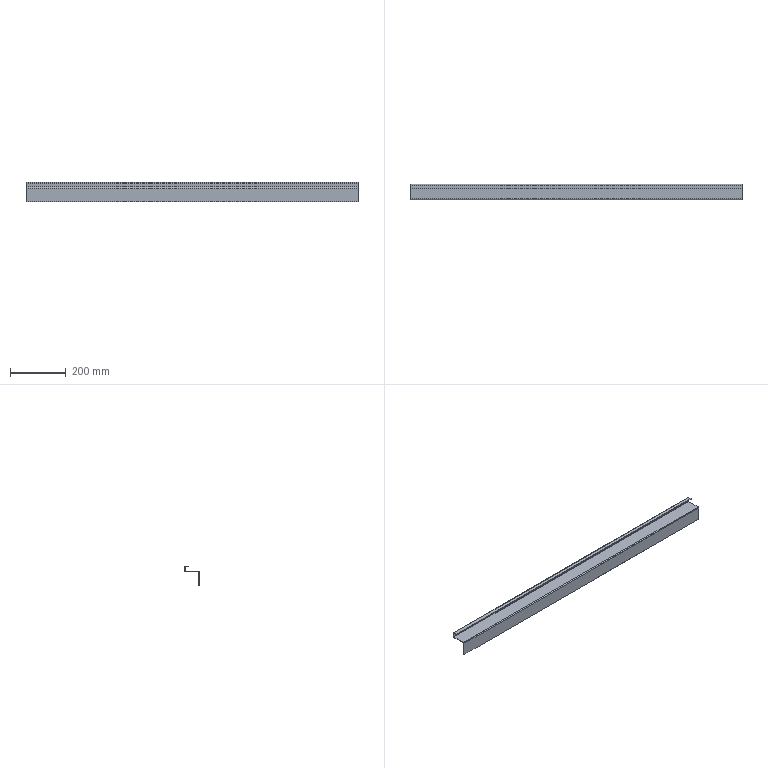Part | SolidWorks | features BaseBody 1 | 1 solid | 30 faces | box 1186 x 54 x 70 mm | volume 314112 mm3 | plane 24 | cylinder 6 | commonest cylinder face diameters 2 x3 6 x3
STEP:
#1=CARTESIAN_POINT('',(-593.,12.,16.));
#2=VERTEX_POINT('',#1);
#3=CARTESIAN_POINT('',(593.,12.,16.));
#4=VERTEX_POINT('',#3);
#5=CARTESIAN_POINT('',(593.,12.,16.));
#6=DIRECTION('',(1.,0.,0.));
#7=VECTOR('',#6,1000.);
#8=LINE('',#5,#7);
#9=EDGE_CURVE('',#2,#4,#8,.T.);
#10=ORIENTED_EDGE('',*,*,#9,.T.);
#11=CARTESIAN_POINT('',(593.,12.,18.));
#12=VERTEX_POINT('',#11);
#13=CARTESIAN_POINT('',(593.,12.,18.));
#14=DIRECTION('',(0.,0.,-1.));
#15=VECTOR('',#14,1000.);
#16=LINE('',#13,#15);
#17=EDGE_CURVE('',#12,#4,#16,.T.);
#18=ORIENTED_EDGE('',*,*,#17,.F.);
#19=CARTESIAN_POINT('',(-593.,12.,18.));
#20=VERTEX_POINT('',#19);
#21=CARTESIAN_POINT('',(0.,12.,18.));
#22=DIRECTION('',(1.,0.,0.));
#23=VECTOR('',#22,1000.);
#24=LINE('',#21,#23);
#25=EDGE_CURVE('',#20,#12,#24,.T.);
#26=ORIENTED_EDGE('',*,*,#25,.F.);
#27=CARTESIAN_POINT('',(-593.,12.,18.));
#28=DIRECTION('',(0.,0.,-1.));
#29=VECTOR('',#28,1000.);
#30=LINE('',#27,#29);
#31=EDGE_CURVE('',#20,#2,#30,.T.);
#32=ORIENTED_EDGE('',*,*,#31,.T.);
#33=EDGE_LOOP('',(#10,#18,#26,#32));
#34=FACE_OUTER_BOUND('',#33,.T.);
#35=CARTESIAN_POINT('',(593.,12.,18.));
#36=DIRECTION('',(0.,1.,0.));
#37=DIRECTION('',(0.,0.,-1.));
#38=AXIS2_PLACEMENT_3D('',#35,#36,#37);
#39=PLANE('',#38);
#40=ADVANCED_FACE('',(#34),#39,.F.);
#41=CARTESIAN_POINT('',(-593.,24.,16.));
#42=VERTEX_POINT('',#41);
#43=CARTESIAN_POINT('',(-593.,12.,16.));
#44=DIRECTION('',(0.,-1.,0.));
#45=VECTOR('',#44,1000.);
#46=LINE('',#43,#45);
#47=EDGE_CURVE('',#42,#2,#46,.T.);
#48=ORIENTED_EDGE('',*,*,#47,.F.);
#49=CARTESIAN_POINT('',(593.,24.,16.));
#50=VERTEX_POINT('',#49);
#51=CARTESIAN_POINT('',(593.,24.,16.));
#52=DIRECTION('',(-1.,0.,0.));
#53=VECTOR('',#52,1000.);
#54=LINE('',#51,#53);
#55=EDGE_CURVE('',#50,#42,#54,.T.);
#56=ORIENTED_EDGE('',*,*,#55,.F.);
#57=CARTESIAN_POINT('',(593.,25.,16.));
#58=DIRECTION('',(0.,1.,0.));
#59=VECTOR('',#58,1000.);
#60=LINE('',#57,#59);
#61=EDGE_CURVE('',#4,#50,#60,.T.);
#62=ORIENTED_EDGE('',*,*,#61,.F.);
#63=ORIENTED_EDGE('',*,*,#9,.F.);
#64=EDGE_LOOP('',(#48,#56,#62,#63));
#65=FACE_OUTER_BOUND('',#64,.T.);
#66=CARTESIAN_POINT('',(0.,0.,16.));
#67=DIRECTION('',(0.,0.,-1.));
#68=DIRECTION('',(0.,-1.,0.));
#69=AXIS2_PLACEMENT_3D('',#66,#67,#68);
#70=PLANE('',#69);
#71=ADVANCED_FACE('',(#65),#70,.T.);
#72=CARTESIAN_POINT('',(-593.,24.,18.));
#73=VERTEX_POINT('',#72);
#74=CARTESIAN_POINT('',(593.,24.,18.));
#75=VERTEX_POINT('',#74);
#76=CARTESIAN_POINT('',(593.,24.,18.));
#77=DIRECTION('',(1.,0.,0.));
#78=VECTOR('',#77,1000.);
#79=LINE('',#76,#78);
#80=EDGE_CURVE('',#73,#75,#79,.T.);
#81=ORIENTED_EDGE('',*,*,#80,.F.);
#82=CARTESIAN_POINT('',(-593.,0.,18.));
#83=DIRECTION('',(0.,-1.,0.));
#84=VECTOR('',#83,1000.);
#85=LINE('',#82,#84);
#86=EDGE_CURVE('',#73,#20,#85,.T.);
#87=ORIENTED_EDGE('',*,*,#86,.T.);
#88=ORIENTED_EDGE('',*,*,#25,.T.);
#89=CARTESIAN_POINT('',(593.,0.,18.));
#90=DIRECTION('',(0.,1.,0.));
#91=VECTOR('',#90,1000.);
#92=LINE('',#89,#91);
#93=EDGE_CURVE('',#12,#75,#92,.T.);
#94=ORIENTED_EDGE('',*,*,#93,.T.);
#95=EDGE_LOOP('',(#81,#87,#88,#94));
#96=FACE_OUTER_BOUND('',#95,.T.);
#97=CARTESIAN_POINT('',(0.,0.,18.));
#98=DIRECTION('',(0.,0.,-1.));
#99=DIRECTION('',(0.,-1.,0.));
#100=AXIS2_PLACEMENT_3D('',#97,#98,#99);
#101=PLANE('',#100);
#102=ADVANCED_FACE('',(#96),#101,.F.);
#103=CARTESIAN_POINT('',(-593.,24.,16.));
#104=DIRECTION('',(0.,0.,1.));
#105=VECTOR('',#104,1000.);
#106=LINE('',#103,#105);
#107=EDGE_CURVE('',#42,#73,#106,.T.);
#108=ORIENTED_EDGE('',*,*,#107,.F.);
#109=ORIENTED_EDGE('',*,*,#47,.T.);
#110=ORIENTED_EDGE('',*,*,#31,.F.);
#111=ORIENTED_EDGE('',*,*,#86,.F.);
#112=EDGE_LOOP('',(#108,#109,#110,#111));
#113=FACE_OUTER_BOUND('',#112,.T.);
#114=CARTESIAN_POINT('',(-593.,12.,18.));
#115=DIRECTION('',(1.,0.,0.));
#116=DIRECTION('',(0.,0.,1.));
#117=AXIS2_PLACEMENT_3D('',#114,#115,#116);
#118=PLANE('',#117);
#119=ADVANCED_FACE('',(#113),#118,.F.);
#120=CARTESIAN_POINT('',(593.,24.,18.));
#121=DIRECTION('',(0.,0.,1.));
#122=VECTOR('',#121,1000.);
#123=LINE('',#120,#122);
#124=EDGE_CURVE('',#50,#75,#123,.T.);
#125=ORIENTED_EDGE('',*,*,#124,.T.);
#126=ORIENTED_EDGE('',*,*,#93,.F.);
#127=ORIENTED_EDGE('',*,*,#17,.T.);
#128=ORIENTED_EDGE('',*,*,#61,.T.);
#129=EDGE_LOOP('',(#125,#126,#127,#128));
#130=FACE_OUTER_BOUND('',#129,.T.);
#131=CARTESIAN_POINT('',(593.,25.,18.));
#132=DIRECTION('',(-1.,0.,0.));
#133=DIRECTION('',(0.,0.,1.));
#134=AXIS2_PLACEMENT_3D('',#131,#132,#133);
#135=PLANE('',#134);
#136=ADVANCED_FACE('',(#130),#135,.F.);
#137=CARTESIAN_POINT('',(-593.,25.,15.));
#138=VERTEX_POINT('',#137);
#139=CARTESIAN_POINT('',(593.,25.,15.));
#140=VERTEX_POINT('',#139);
#141=CARTESIAN_POINT('',(-593.,25.,15.));
#142=DIRECTION('',(1.,0.,0.));
#143=VECTOR('',#142,1000.);
#144=LINE('',#141,#143);
#145=EDGE_CURVE('',#138,#140,#144,.T.);
#146=ORIENTED_EDGE('',*,*,#145,.T.);
#147=CARTESIAN_POINT('',(593.,24.,15.));
#148=DIRECTION('',(1.,0.,0.));
#149=DIRECTION('',(0.,0.,1.));
#150=AXIS2_PLACEMENT_3D('',#147,#148,#149);
#151=CIRCLE('',#150,1.);
#152=EDGE_CURVE('',#140,#50,#151,.T.);
#153=ORIENTED_EDGE('',*,*,#152,.T.);
#154=ORIENTED_EDGE('',*,*,#55,.T.);
#155=CARTESIAN_POINT('',(-593.,24.,15.));
#156=DIRECTION('',(-1.,0.,0.));
#157=DIRECTION('',(0.,0.,1.));
#158=AXIS2_PLACEMENT_3D('',#155,#156,#157);
#159=CIRCLE('',#158,1.);
#160=EDGE_CURVE('',#42,#138,#159,.T.);
#161=ORIENTED_EDGE('',*,*,#160,.T.);
#162=EDGE_LOOP('',(#146,#153,#154,#161));
#163=FACE_OUTER_BOUND('',#162,.T.);
#164=CARTESIAN_POINT('',(-593.,24.,15.));
#165=DIRECTION('',(-1.,0.,0.));
#166=DIRECTION('',(0.,0.,1.));
#167=AXIS2_PLACEMENT_3D('',#164,#165,#166);
#168=CYLINDRICAL_SURFACE('',#167,1.);
#169=ADVANCED_FACE('',(#163),#168,.F.);
#170=CARTESIAN_POINT('',(-593.,27.,15.));
#171=VERTEX_POINT('',#170);
#172=CARTESIAN_POINT('',(593.,27.,15.));
#173=VERTEX_POINT('',#172);
#174=CARTESIAN_POINT('',(-593.,27.,15.));
#175=DIRECTION('',(1.,0.,0.));
#176=VECTOR('',#175,1000.);
#177=LINE('',#174,#176);
#178=EDGE_CURVE('',#171,#173,#177,.T.);
#179=ORIENTED_EDGE('',*,*,#178,.F.);
#180=CARTESIAN_POINT('',(-593.,24.,15.));
#181=DIRECTION('',(-1.,0.,0.));
#182=DIRECTION('',(0.,0.,1.));
#183=AXIS2_PLACEMENT_3D('',#180,#181,#182);
#184=CIRCLE('',#183,3.);
#185=EDGE_CURVE('',#73,#171,#184,.T.);
#186=ORIENTED_EDGE('',*,*,#185,.F.);
#187=ORIENTED_EDGE('',*,*,#80,.T.);
#188=CARTESIAN_POINT('',(593.,24.,15.));
#189=DIRECTION('',(1.,0.,0.));
#190=DIRECTION('',(0.,0.,1.));
#191=AXIS2_PLACEMENT_3D('',#188,#189,#190);
#192=CIRCLE('',#191,3.);
#193=EDGE_CURVE('',#173,#75,#192,.T.);
#194=ORIENTED_EDGE('',*,*,#193,.F.);
#195=EDGE_LOOP('',(#179,#186,#187,#194));
#196=FACE_OUTER_BOUND('',#195,.T.);
#197=CARTESIAN_POINT('',(-593.,24.,15.));
#198=DIRECTION('',(-1.,0.,0.));
#199=DIRECTION('',(0.,0.,1.));
#200=AXIS2_PLACEMENT_3D('',#197,#198,#199);
#201=CYLINDRICAL_SURFACE('',#200,3.);
#202=ADVANCED_FACE('',(#196),#201,.T.);
#203=ORIENTED_EDGE('',*,*,#160,.F.);
#204=ORIENTED_EDGE('',*,*,#107,.T.);
#205=ORIENTED_EDGE('',*,*,#185,.T.);
#206=CARTESIAN_POINT('',(-593.,25.,15.));
#207=DIRECTION('',(0.,1.,0.));
#208=VECTOR('',#207,1000.);
#209=LINE('',#206,#208);
#210=EDGE_CURVE('',#138,#171,#209,.T.);
#211=ORIENTED_EDGE('',*,*,#210,.F.);
#212=EDGE_LOOP('',(#203,#204,#205,#211));
#213=FACE_OUTER_BOUND('',#212,.T.);
#214=CARTESIAN_POINT('',(-593.,24.,15.));
#215=DIRECTION('',(1.,0.,0.));
#216=DIRECTION('',(0.,1.,0.));
#217=AXIS2_PLACEMENT_3D('',#214,#215,#216);
#218=PLANE('',#217);
#219=ADVANCED_FACE('',(#213),#218,.F.);
#220=ORIENTED_EDGE('',*,*,#124,.F.);
#221=ORIENTED_EDGE('',*,*,#152,.F.);
#222=CARTESIAN_POINT('',(593.,25.,15.));
#223=DIRECTION('',(0.,1.,0.));
#224=VECTOR('',#223,1000.);
#225=LINE('',#222,#224);
#226=EDGE_CURVE('',#140,#173,#225,.T.);
#227=ORIENTED_EDGE('',*,*,#226,.T.);
#228=ORIENTED_EDGE('',*,*,#193,.T.);
#229=EDGE_LOOP('',(#220,#221,#227,#228));
#230=FACE_OUTER_BOUND('',#229,.T.);
#231=CARTESIAN_POINT('',(593.,24.,15.));
#232=DIRECTION('',(1.,0.,0.));
#233=DIRECTION('',(0.,1.,0.));
#234=AXIS2_PLACEMENT_3D('',#231,#232,#233);
#235=PLANE('',#234);
#236=ADVANCED_FACE('',(#230),#235,.T.);
#237=ORIENTED_EDGE('',*,*,#226,.F.);
#238=CARTESIAN_POINT('',(593.,25.,1.));
#239=VERTEX_POINT('',#238);
#240=CARTESIAN_POINT('',(593.,25.,0.));
#241=DIRECTION('',(0.,0.,1.));
#242=VECTOR('',#241,1000.);
#243=LINE('',#240,#242);
#244=EDGE_CURVE('',#239,#140,#243,.T.);
#245=ORIENTED_EDGE('',*,*,#244,.F.);
#246=CARTESIAN_POINT('',(593.,27.,1.));
#247=VERTEX_POINT('',#246);
#248=CARTESIAN_POINT('',(593.,27.,1.));
#249=DIRECTION('',(0.,1.,0.));
#250=VECTOR('',#249,1000.);
#251=LINE('',#248,#250);
#252=EDGE_CURVE('',#239,#247,#251,.T.);
#253=ORIENTED_EDGE('',*,*,#252,.T.);
#254=CARTESIAN_POINT('',(593.,27.,18.));
#255=DIRECTION('',(0.,0.,1.));
#256=VECTOR('',#255,1000.);
#257=LINE('',#254,#256);
#258=EDGE_CURVE('',#247,#173,#257,.T.);
#259=ORIENTED_EDGE('',*,*,#258,.T.);
#260=EDGE_LOOP('',(#237,#245,#253,#259));
#261=FACE_OUTER_BOUND('',#260,.T.);
#262=CARTESIAN_POINT('',(593.,27.,18.));
#263=DIRECTION('',(1.,0.,0.));
#264=DIRECTION('',(0.,1.,0.));
#265=AXIS2_PLACEMENT_3D('',#262,#263,#264);
#266=PLANE('',#265);
#267=ADVANCED_FACE('',(#261),#266,.T.);
#268=CARTESIAN_POINT('',(-593.,24.,0.));
#269=VERTEX_POINT('',#268);
#270=CARTESIAN_POINT('',(593.,24.,0.));
#271=VERTEX_POINT('',#270);
#272=CARTESIAN_POINT('',(-593.,24.,0.));
#273=DIRECTION('',(1.,0.,0.));
#274=VECTOR('',#273,1000.);
#275=LINE('',#272,#274);
#276=EDGE_CURVE('',#269,#271,#275,.T.);
#277=ORIENTED_EDGE('',*,*,#276,.T.);
#278=CARTESIAN_POINT('',(593.,24.,1.));
#279=DIRECTION('',(1.,0.,0.));
#280=DIRECTION('',(0.,0.,1.));
#281=AXIS2_PLACEMENT_3D('',#278,#279,#280);
#282=CIRCLE('',#281,1.);
#283=EDGE_CURVE('',#271,#239,#282,.T.);
#284=ORIENTED_EDGE('',*,*,#283,.T.);
#285=CARTESIAN_POINT('',(-593.,25.,1.));
#286=VERTEX_POINT('',#285);
#287=CARTESIAN_POINT('',(593.,25.,1.));
#288=DIRECTION('',(-1.,0.,0.));
#289=VECTOR('',#288,1000.);
#290=LINE('',#287,#289);
#291=EDGE_CURVE('',#239,#286,#290,.T.);
#292=ORIENTED_EDGE('',*,*,#291,.T.);
#293=CARTESIAN_POINT('',(-593.,24.,1.));
#294=DIRECTION('',(-1.,0.,0.));
#295=DIRECTION('',(0.,0.,1.));
#296=AXIS2_PLACEMENT_3D('',#293,#294,#295);
#297=CIRCLE('',#296,1.);
#298=EDGE_CURVE('',#286,#269,#297,.T.);
#299=ORIENTED_EDGE('',*,*,#298,.T.);
#300=EDGE_LOOP('',(#277,#284,#292,#299));
#301=FACE_OUTER_BOUND('',#300,.T.);
#302=CARTESIAN_POINT('',(-593.,24.,1.));
#303=DIRECTION('',(-1.,0.,0.));
#304=DIRECTION('',(0.,1.,0.));
#305=AXIS2_PLACEMENT_3D('',#302,#303,#304);
#306=CYLINDRICAL_SURFACE('',#305,1.);
#307=ADVANCED_FACE('',(#301),#306,.F.);
#308=CARTESIAN_POINT('',(-593.,24.,-2.));
#309=VERTEX_POINT('',#308);
#310=CARTESIAN_POINT('',(593.,24.,-2.));
#311=VERTEX_POINT('',#310);
#312=CARTESIAN_POINT('',(-593.,24.,-2.));
#313=DIRECTION('',(1.,0.,0.));
#314=VECTOR('',#313,1000.);
#315=LINE('',#312,#314);
#316=EDGE_CURVE('',#309,#311,#315,.T.);
#317=ORIENTED_EDGE('',*,*,#316,.F.);
#318=CARTESIAN_POINT('',(-593.,27.,1.));
#319=VERTEX_POINT('',#318);
#320=CARTESIAN_POINT('',(-593.,24.,1.));
#321=DIRECTION('',(-1.,0.,0.));
#322=DIRECTION('',(0.,0.,1.));
#323=AXIS2_PLACEMENT_3D('',#320,#321,#322);
#324=CIRCLE('',#323,3.);
#325=EDGE_CURVE('',#319,#309,#324,.T.);
#326=ORIENTED_EDGE('',*,*,#325,.F.);
#327=CARTESIAN_POINT('',(0.,27.,1.));
#328=DIRECTION('',(-1.,0.,0.));
#329=VECTOR('',#328,1000.);
#330=LINE('',#327,#329);
#331=EDGE_CURVE('',#247,#319,#330,.T.);
#332=ORIENTED_EDGE('',*,*,#331,.F.);
#333=CARTESIAN_POINT('',(593.,24.,1.));
#334=DIRECTION('',(1.,0.,0.));
#335=DIRECTION('',(0.,0.,1.));
#336=AXIS2_PLACEMENT_3D('',#333,#334,#335);
#337=CIRCLE('',#336,3.);
#338=EDGE_CURVE('',#311,#247,#337,.T.);
#339=ORIENTED_EDGE('',*,*,#338,.F.);
#340=EDGE_LOOP('',(#317,#326,#332,#339));
#341=FACE_OUTER_BOUND('',#340,.T.);
#342=CARTESIAN_POINT('',(-593.,24.,1.));
#343=DIRECTION('',(-1.,0.,0.));
#344=DIRECTION('',(0.,1.,0.));
#345=AXIS2_PLACEMENT_3D('',#342,#343,#344);
#346=CYLINDRICAL_SURFACE('',#345,3.);
#347=ADVANCED_FACE('',(#341),#346,.T.);
#348=ORIENTED_EDGE('',*,*,#298,.F.);
#349=CARTESIAN_POINT('',(-593.,25.,1.));
#350=DIRECTION('',(0.,1.,0.));
#351=VECTOR('',#350,1000.);
#352=LINE('',#349,#351);
#353=EDGE_CURVE('',#286,#319,#352,.T.);
#354=ORIENTED_EDGE('',*,*,#353,.T.);
#355=ORIENTED_EDGE('',*,*,#325,.T.);
#356=CARTESIAN_POINT('',(-593.,24.,0.));
#357=DIRECTION('',(0.,0.,-1.));
#358=VECTOR('',#357,1000.);
#359=LINE('',#356,#358);
#360=EDGE_CURVE('',#269,#309,#359,.T.);
#361=ORIENTED_EDGE('',*,*,#360,.F.);
#362=EDGE_LOOP('',(#348,#354,#355,#361));
#363=FACE_OUTER_BOUND('',#362,.T.);
#364=CARTESIAN_POINT('',(-593.,24.,1.));
#365=DIRECTION('',(1.,0.,0.));
#366=DIRECTION('',(0.,1.,0.));
#367=AXIS2_PLACEMENT_3D('',#364,#365,#366);
#368=PLANE('',#367);
#369=ADVANCED_FACE('',(#363),#368,.F.);
#370=ORIENTED_EDGE('',*,*,#252,.F.);
#371=ORIENTED_EDGE('',*,*,#283,.F.);
#372=CARTESIAN_POINT('',(593.,24.,0.));
#373=DIRECTION('',(0.,0.,-1.));
#374=VECTOR('',#373,1000.);
#375=LINE('',#372,#374);
#376=EDGE_CURVE('',#271,#311,#375,.T.);
#377=ORIENTED_EDGE('',*,*,#376,.T.);
#378=ORIENTED_EDGE('',*,*,#338,.T.);
#379=EDGE_LOOP('',(#370,#371,#377,#378));
#380=FACE_OUTER_BOUND('',#379,.T.);
#381=CARTESIAN_POINT('',(593.,24.,1.));
#382=DIRECTION('',(1.,0.,0.));
#383=DIRECTION('',(0.,1.,0.));
#384=AXIS2_PLACEMENT_3D('',#381,#382,#383);
#385=PLANE('',#384);
#386=ADVANCED_FACE('',(#380),#385,.T.);
#387=CARTESIAN_POINT('',(-593.,-25.,-52.));
#388=VERTEX_POINT('',#387);
#389=CARTESIAN_POINT('',(593.,-25.,-52.));
#390=VERTEX_POINT('',#389);
#391=CARTESIAN_POINT('',(593.,-25.,-52.));
#392=DIRECTION('',(1.,0.,0.));
#393=VECTOR('',#392,1000.);
#394=LINE('',#391,#393);
#395=EDGE_CURVE('',#388,#390,#394,.T.);
#396=ORIENTED_EDGE('',*,*,#395,.T.);
#397=CARTESIAN_POINT('',(593.,-27.,-52.));
#398=VERTEX_POINT('',#397);
#399=CARTESIAN_POINT('',(593.,-27.,-52.));
#400=DIRECTION('',(0.,1.,0.));
#401=VECTOR('',#400,1000.);
#402=LINE('',#399,#401);
#403=EDGE_CURVE('',#398,#390,#402,.T.);
#404=ORIENTED_EDGE('',*,*,#403,.F.);
#405=CARTESIAN_POINT('',(-593.,-27.,-52.));
#406=VERTEX_POINT('',#405);
#407=CARTESIAN_POINT('',(0.,-27.,-52.));
#408=DIRECTION('',(1.,0.,0.));
#409=VECTOR('',#408,1000.);
#410=LINE('',#407,#409);
#411=EDGE_CURVE('',#406,#398,#410,.T.);
#412=ORIENTED_EDGE('',*,*,#411,.F.);
#413=CARTESIAN_POINT('',(-593.,-27.,-52.));
#414=DIRECTION('',(0.,1.,0.));
#415=VECTOR('',#414,1000.);
#416=LINE('',#413,#415);
#417=EDGE_CURVE('',#406,#388,#416,.T.);
#418=ORIENTED_EDGE('',*,*,#417,.T.);
#419=EDGE_LOOP('',(#396,#404,#412,#418));
#420=FACE_OUTER_BOUND('',#419,.T.);
#421=CARTESIAN_POINT('',(593.,-27.,-52.));
#422=DIRECTION('',(0.,0.,1.));
#423=DIRECTION('',(0.,-1.,0.));
#424=AXIS2_PLACEMENT_3D('',#421,#422,#423);
#425=PLANE('',#424);
#426=ADVANCED_FACE('',(#420),#425,.F.);
#427=CARTESIAN_POINT('',(-593.,-25.,-3.));
#428=VERTEX_POINT('',#427);
#429=CARTESIAN_POINT('',(-593.,-25.,-52.));
#430=DIRECTION('',(0.,0.,-1.));
#431=VECTOR('',#430,1000.);
#432=LINE('',#429,#431);
#433=EDGE_CURVE('',#428,#388,#432,.T.);
#434=ORIENTED_EDGE('',*,*,#433,.F.);
#435=CARTESIAN_POINT('',(593.,-25.,-3.));
#436=VERTEX_POINT('',#435);
#437=CARTESIAN_POINT('',(593.,-25.,-3.));
#438=DIRECTION('',(-1.,0.,0.));
#439=VECTOR('',#438,1000.);
#440=LINE('',#437,#439);
#441=EDGE_CURVE('',#436,#428,#440,.T.);
#442=ORIENTED_EDGE('',*,*,#441,.F.);
#443=CARTESIAN_POINT('',(593.,-25.,-2.));
#444=DIRECTION('',(0.,0.,1.));
#445=VECTOR('',#444,1000.);
#446=LINE('',#443,#445);
#447=EDGE_CURVE('',#390,#436,#446,.T.);
#448=ORIENTED_EDGE('',*,*,#447,.F.);
#449=ORIENTED_EDGE('',*,*,#395,.F.);
#450=EDGE_LOOP('',(#434,#442,#448,#449));
#451=FACE_OUTER_BOUND('',#450,.T.);
#452=CARTESIAN_POINT('',(0.,-25.,0.));
#453=DIRECTION('',(0.,1.,0.));
#454=DIRECTION('',(0.,0.,-1.));
#455=AXIS2_PLACEMENT_3D('',#452,#453,#454);
#456=PLANE('',#455);
#457=ADVANCED_FACE('',(#451),#456,.T.);
#458=CARTESIAN_POINT('',(-593.,-27.,-3.));
#459=VERTEX_POINT('',#458);
#460=CARTESIAN_POINT('',(593.,-27.,-3.));
#461=VERTEX_POINT('',#460);
#462=CARTESIAN_POINT('',(593.,-27.,-3.));
#463=DIRECTION('',(1.,0.,0.));
#464=VECTOR('',#463,1000.);
#465=LINE('',#462,#464);
#466=EDGE_CURVE('',#459,#461,#465,.T.);
#467=ORIENTED_EDGE('',*,*,#466,.F.);
#468=CARTESIAN_POINT('',(-593.,-27.,0.));
#469=DIRECTION('',(0.,0.,-1.));
#470=VECTOR('',#469,1000.);
#471=LINE('',#468,#470);
#472=EDGE_CURVE('',#459,#406,#471,.T.);
#473=ORIENTED_EDGE('',*,*,#472,.T.);
#474=ORIENTED_EDGE('',*,*,#411,.T.);
#475=CARTESIAN_POINT('',(593.,-27.,0.));
#476=DIRECTION('',(0.,0.,1.));
#477=VECTOR('',#476,1000.);
#478=LINE('',#475,#477);
#479=EDGE_CURVE('',#398,#461,#478,.T.);
#480=ORIENTED_EDGE('',*,*,#479,.T.);
#481=EDGE_LOOP('',(#467,#473,#474,#480));
#482=FACE_OUTER_BOUND('',#481,.T.);
#483=CARTESIAN_POINT('',(0.,-27.,0.));
#484=DIRECTION('',(0.,1.,0.));
#485=DIRECTION('',(0.,0.,-1.));
#486=AXIS2_PLACEMENT_3D('',#483,#484,#485);
#487=PLANE('',#486);
#488=ADVANCED_FACE('',(#482),#487,.F.);
#489=CARTESIAN_POINT('',(593.,-27.,-3.));
#490=DIRECTION('',(0.,-1.,0.));
#491=VECTOR('',#490,1000.);
#492=LINE('',#489,#491);
#493=EDGE_CURVE('',#436,#461,#492,.T.);
#494=ORIENTED_EDGE('',*,*,#493,.T.);
#495=ORIENTED_EDGE('',*,*,#479,.F.);
#496=ORIENTED_EDGE('',*,*,#403,.T.);
#497=ORIENTED_EDGE('',*,*,#447,.T.);
#498=EDGE_LOOP('',(#494,#495,#496,#497));
#499=FACE_OUTER_BOUND('',#498,.T.);
#500=CARTESIAN_POINT('',(593.,-27.,-2.));
#501=DIRECTION('',(-1.,0.,0.));
#502=DIRECTION('',(0.,1.,0.));
#503=AXIS2_PLACEMENT_3D('',#500,#501,#502);
#504=PLANE('',#503);
#505=ADVANCED_FACE('',(#499),#504,.F.);
#506=CARTESIAN_POINT('',(-593.,-25.,-3.));
#507=DIRECTION('',(0.,-1.,0.));
#508=VECTOR('',#507,1000.);
#509=LINE('',#506,#508);
#510=EDGE_CURVE('',#428,#459,#509,.T.);
#511=ORIENTED_EDGE('',*,*,#510,.F.);
#512=ORIENTED_EDGE('',*,*,#433,.T.);
#513=ORIENTED_EDGE('',*,*,#417,.F.);
#514=ORIENTED_EDGE('',*,*,#472,.F.);
#515=EDGE_LOOP('',(#511,#512,#513,#514));
#516=FACE_OUTER_BOUND('',#515,.T.);
#517=CARTESIAN_POINT('',(-593.,-27.,-52.));
#518=DIRECTION('',(1.,0.,0.));
#519=DIRECTION('',(0.,1.,0.));
#520=AXIS2_PLACEMENT_3D('',#517,#518,#519);
#521=PLANE('',#520);
#522=ADVANCED_FACE('',(#516),#521,.F.);
#523=CARTESIAN_POINT('',(-593.,-24.,-2.));
#524=VERTEX_POINT('',#523);
#525=CARTESIAN_POINT('',(593.,-24.,-2.));
#526=VERTEX_POINT('',#525);
#527=CARTESIAN_POINT('',(-593.,-24.,-2.));
#528=DIRECTION('',(1.,0.,0.));
#529=VECTOR('',#528,1000.);
#530=LINE('',#527,#529);
#531=EDGE_CURVE('',#524,#526,#530,.T.);
#532=ORIENTED_EDGE('',*,*,#531,.T.);
#533=CARTESIAN_POINT('',(593.,-24.,-3.));
#534=DIRECTION('',(1.,0.,0.));
#535=DIRECTION('',(0.,0.,1.));
#536=AXIS2_PLACEMENT_3D('',#533,#534,#535);
#537=CIRCLE('',#536,1.);
#538=EDGE_CURVE('',#526,#436,#537,.T.);
#539=ORIENTED_EDGE('',*,*,#538,.T.);
#540=ORIENTED_EDGE('',*,*,#441,.T.);
#541=CARTESIAN_POINT('',(-593.,-24.,-3.));
#542=DIRECTION('',(-1.,0.,0.));
#543=DIRECTION('',(0.,0.,1.));
#544=AXIS2_PLACEMENT_3D('',#541,#542,#543);
#545=CIRCLE('',#544,1.);
#546=EDGE_CURVE('',#428,#524,#545,.T.);
#547=ORIENTED_EDGE('',*,*,#546,.T.);
#548=EDGE_LOOP('',(#532,#539,#540,#547));
#549=FACE_OUTER_BOUND('',#548,.T.);
#550=CARTESIAN_POINT('',(-593.,-24.,-3.));
#551=DIRECTION('',(-1.,0.,0.));
#552=DIRECTION('',(0.,-1.,0.));
#553=AXIS2_PLACEMENT_3D('',#550,#551,#552);
#554=CYLINDRICAL_SURFACE('',#553,1.);
#555=ADVANCED_FACE('',(#549),#554,.F.);
#556=CARTESIAN_POINT('',(-593.,-24.,0.));
#557=VERTEX_POINT('',#556);
#558=CARTESIAN_POINT('',(593.,-24.,0.));
#559=VERTEX_POINT('',#558);
#560=CARTESIAN_POINT('',(-593.,-24.,0.));
#561=DIRECTION('',(1.,0.,0.));
#562=VECTOR('',#561,1000.);
#563=LINE('',#560,#562);
#564=EDGE_CURVE('',#557,#559,#563,.T.);
#565=ORIENTED_EDGE('',*,*,#564,.F.);
#566=CARTESIAN_POINT('',(-593.,-24.,-3.));
#567=DIRECTION('',(-1.,0.,0.));
#568=DIRECTION('',(0.,0.,1.));
#569=AXIS2_PLACEMENT_3D('',#566,#567,#568);
#570=CIRCLE('',#569,3.);
#571=EDGE_CURVE('',#459,#557,#570,.T.);
#572=ORIENTED_EDGE('',*,*,#571,.F.);
#573=ORIENTED_EDGE('',*,*,#466,.T.);
#574=CARTESIAN_POINT('',(593.,-24.,-3.));
#575=DIRECTION('',(1.,0.,0.));
#576=DIRECTION('',(0.,0.,1.));
#577=AXIS2_PLACEMENT_3D('',#574,#575,#576);
#578=CIRCLE('',#577,3.);
#579=EDGE_CURVE('',#559,#461,#578,.T.);
#580=ORIENTED_EDGE('',*,*,#579,.F.);
#581=EDGE_LOOP('',(#565,#572,#573,#580));
#582=FACE_OUTER_BOUND('',#581,.T.);
#583=CARTESIAN_POINT('',(-593.,-24.,-3.));
#584=DIRECTION('',(-1.,0.,0.));
#585=DIRECTION('',(0.,-1.,0.));
#586=AXIS2_PLACEMENT_3D('',#583,#584,#585);
#587=CYLINDRICAL_SURFACE('',#586,3.);
#588=ADVANCED_FACE('',(#582),#587,.T.);
#589=ORIENTED_EDGE('',*,*,#546,.F.);
#590=ORIENTED_EDGE('',*,*,#510,.T.);
#591=ORIENTED_EDGE('',*,*,#571,.T.);
#592=CARTESIAN_POINT('',(-593.,-24.,-2.));
#593=DIRECTION('',(0.,0.,1.));
#594=VECTOR('',#593,1000.);
#595=LINE('',#592,#594);
#596=EDGE_CURVE('',#524,#557,#595,.T.);
#597=ORIENTED_EDGE('',*,*,#596,.F.);
#598=EDGE_LOOP('',(#589,#590,#591,#597));
#599=FACE_OUTER_BOUND('',#598,.T.);
#600=CARTESIAN_POINT('',(-593.,-24.,-3.));
#601=DIRECTION('',(1.,0.,0.));
#602=DIRECTION('',(0.,1.,0.));
#603=AXIS2_PLACEMENT_3D('',#600,#601,#602);
#604=PLANE('',#603);
#605=ADVANCED_FACE('',(#599),#604,.F.);
#606=ORIENTED_EDGE('',*,*,#493,.F.);
#607=ORIENTED_EDGE('',*,*,#538,.F.);
#608=CARTESIAN_POINT('',(593.,-24.,-2.));
#609=DIRECTION('',(0.,0.,1.));
#610=VECTOR('',#609,1000.);
#611=LINE('',#608,#610);
#612=EDGE_CURVE('',#526,#559,#611,.T.);
#613=ORIENTED_EDGE('',*,*,#612,.T.);
#614=ORIENTED_EDGE('',*,*,#579,.T.);
#615=EDGE_LOOP('',(#606,#607,#613,#614));
#616=FACE_OUTER_BOUND('',#615,.T.);
#617=CARTESIAN_POINT('',(593.,-24.,-3.));
#618=DIRECTION('',(1.,0.,0.));
#619=DIRECTION('',(0.,1.,0.));
#620=AXIS2_PLACEMENT_3D('',#617,#618,#619);
#621=PLANE('',#620);
#622=ADVANCED_FACE('',(#616),#621,.T.);
#623=ORIENTED_EDGE('',*,*,#376,.F.);
#624=CARTESIAN_POINT('',(593.,27.,0.));
#625=DIRECTION('',(0.,1.,0.));
#626=VECTOR('',#625,1000.);
#627=LINE('',#624,#626);
#628=EDGE_CURVE('',#559,#271,#627,.T.);
#629=ORIENTED_EDGE('',*,*,#628,.F.);
#630=ORIENTED_EDGE('',*,*,#612,.F.);
#631=CARTESIAN_POINT('',(593.,27.,-2.));
#632=DIRECTION('',(0.,1.,0.));
#633=VECTOR('',#632,1000.);
#634=LINE('',#631,#633);
#635=EDGE_CURVE('',#526,#311,#634,.T.);
#636=ORIENTED_EDGE('',*,*,#635,.T.);
#637=EDGE_LOOP('',(#623,#629,#630,#636));
#638=FACE_OUTER_BOUND('',#637,.T.);
#639=CARTESIAN_POINT('',(593.,27.,-2.));
#640=DIRECTION('',(1.,0.,0.));
#641=DIRECTION('',(0.,-1.,0.));
#642=AXIS2_PLACEMENT_3D('',#639,#640,#641);
#643=PLANE('',#642);
#644=ADVANCED_FACE('',(#638),#643,.T.);
#645=ORIENTED_EDGE('',*,*,#276,.F.);
#646=CARTESIAN_POINT('',(-593.,27.,0.));
#647=DIRECTION('',(0.,-1.,0.));
#648=VECTOR('',#647,1000.);
#649=LINE('',#646,#648);
#650=EDGE_CURVE('',#269,#557,#649,.T.);
#651=ORIENTED_EDGE('',*,*,#650,.T.);
#652=ORIENTED_EDGE('',*,*,#564,.T.);
#653=ORIENTED_EDGE('',*,*,#628,.T.);
#654=EDGE_LOOP('',(#645,#651,#652,#653));
#655=FACE_OUTER_BOUND('',#654,.T.);
#656=CARTESIAN_POINT('',(0.,0.,0.));
#657=DIRECTION('',(0.,0.,-1.));
#658=DIRECTION('',(0.,-1.,0.));
#659=AXIS2_PLACEMENT_3D('',#656,#657,#658);
#660=PLANE('',#659);
#661=ADVANCED_FACE('',(#655),#660,.F.);
#662=CARTESIAN_POINT('',(-593.,27.,-2.));
#663=DIRECTION('',(0.,-1.,0.));
#664=VECTOR('',#663,1000.);
#665=LINE('',#662,#664);
#666=EDGE_CURVE('',#309,#524,#665,.T.);
#667=ORIENTED_EDGE('',*,*,#666,.F.);
#668=ORIENTED_EDGE('',*,*,#316,.T.);
#669=ORIENTED_EDGE('',*,*,#635,.F.);
#670=ORIENTED_EDGE('',*,*,#531,.F.);
#671=EDGE_LOOP('',(#667,#668,#669,#670));
#672=FACE_OUTER_BOUND('',#671,.T.);
#673=CARTESIAN_POINT('',(0.,0.,-2.));
#674=DIRECTION('',(0.,0.,-1.));
#675=DIRECTION('',(0.,-1.,0.));
#676=AXIS2_PLACEMENT_3D('',#673,#674,#675);
#677=PLANE('',#676);
#678=ADVANCED_FACE('',(#672),#677,.T.);
#679=ORIENTED_EDGE('',*,*,#650,.F.);
#680=ORIENTED_EDGE('',*,*,#360,.T.);
#681=ORIENTED_EDGE('',*,*,#666,.T.);
#682=ORIENTED_EDGE('',*,*,#596,.T.);
#683=EDGE_LOOP('',(#679,#680,#681,#682));
#684=FACE_OUTER_BOUND('',#683,.T.);
#685=CARTESIAN_POINT('',(-593.,27.,-2.));
#686=DIRECTION('',(-1.,0.,0.));
#687=DIRECTION('',(0.,1.,0.));
#688=AXIS2_PLACEMENT_3D('',#685,#686,#687);
#689=PLANE('',#688);
#690=ADVANCED_FACE('',(#684),#689,.T.);
#691=ORIENTED_EDGE('',*,*,#145,.F.);
#692=CARTESIAN_POINT('',(-593.,25.,0.));
#693=DIRECTION('',(0.,0.,-1.));
#694=VECTOR('',#693,1000.);
#695=LINE('',#692,#694);
#696=EDGE_CURVE('',#138,#286,#695,.T.);
#697=ORIENTED_EDGE('',*,*,#696,.T.);
#698=ORIENTED_EDGE('',*,*,#291,.F.);
#699=ORIENTED_EDGE('',*,*,#244,.T.);
#700=EDGE_LOOP('',(#691,#697,#698,#699));
#701=FACE_OUTER_BOUND('',#700,.T.);
#702=CARTESIAN_POINT('',(0.,25.,0.));
#703=DIRECTION('',(0.,1.,0.));
#704=DIRECTION('',(0.,0.,-1.));
#705=AXIS2_PLACEMENT_3D('',#702,#703,#704);
#706=PLANE('',#705);
#707=ADVANCED_FACE('',(#701),#706,.F.);
#708=CARTESIAN_POINT('',(-593.,27.,0.));
#709=DIRECTION('',(0.,0.,-1.));
#710=VECTOR('',#709,1000.);
#711=LINE('',#708,#710);
#712=EDGE_CURVE('',#171,#319,#711,.T.);
#713=ORIENTED_EDGE('',*,*,#712,.F.);
#714=ORIENTED_EDGE('',*,*,#178,.T.);
#715=ORIENTED_EDGE('',*,*,#258,.F.);
#716=ORIENTED_EDGE('',*,*,#331,.T.);
#717=EDGE_LOOP('',(#713,#714,#715,#716));
#718=FACE_OUTER_BOUND('',#717,.T.);
#719=CARTESIAN_POINT('',(0.,27.,0.));
#720=DIRECTION('',(0.,1.,0.));
#721=DIRECTION('',(0.,0.,-1.));
#722=AXIS2_PLACEMENT_3D('',#719,#720,#721);
#723=PLANE('',#722);
#724=ADVANCED_FACE('',(#718),#723,.T.);
#725=ORIENTED_EDGE('',*,*,#696,.F.);
#726=ORIENTED_EDGE('',*,*,#210,.T.);
#727=ORIENTED_EDGE('',*,*,#712,.T.);
#728=ORIENTED_EDGE('',*,*,#353,.F.);
#729=EDGE_LOOP('',(#725,#726,#727,#728));
#730=FACE_OUTER_BOUND('',#729,.T.);
#731=CARTESIAN_POINT('',(-593.,27.,0.));
#732=DIRECTION('',(-1.,0.,0.));
#733=DIRECTION('',(0.,1.,0.));
#734=AXIS2_PLACEMENT_3D('',#731,#732,#733);
#735=PLANE('',#734);
#736=ADVANCED_FACE('',(#730),#735,.T.);
#737=CLOSED_SHELL('',(#40,#71,#102,#119,#136,#169,#202,#219,#236,#267,#307,#347,#369,#386,#426,#457,#488,#505,#522,#555,#588,#605,#622,#644,#661,#678,#690,#707,#724,#736));
#738=MANIFOLD_SOLID_BREP('',#737);
#739=CARTESIAN_POINT('',(0.,0.,0.));
#740=DIRECTION('',(0.,0.,1.));
#741=DIRECTION('',(1.,0.,0.));
#742=AXIS2_PLACEMENT_3D('',#739,#740,#741);
#743=(LENGTH_UNIT()NAMED_UNIT(*)SI_UNIT(.MILLI.,.METRE.));
#744=UNCERTAINTY_MEASURE_WITH_UNIT(LENGTH_MEASURE(0.00001),#743,'','');
#745=(NAMED_UNIT(*)PLANE_ANGLE_UNIT()SI_UNIT($,.RADIAN.));
#746=(NAMED_UNIT(*)SI_UNIT($,.STERADIAN.)SOLID_ANGLE_UNIT());
#747=(GEOMETRIC_REPRESENTATION_CONTEXT(3)GLOBAL_UNCERTAINTY_ASSIGNED_CONTEXT((#744))GLOBAL_UNIT_ASSIGNED_CONTEXT((#743,#745,#746))REPRESENTATION_CONTEXT('',''));
#748=ADVANCED_BREP_SHAPE_REPRESENTATION('',(#738,#742),#747);